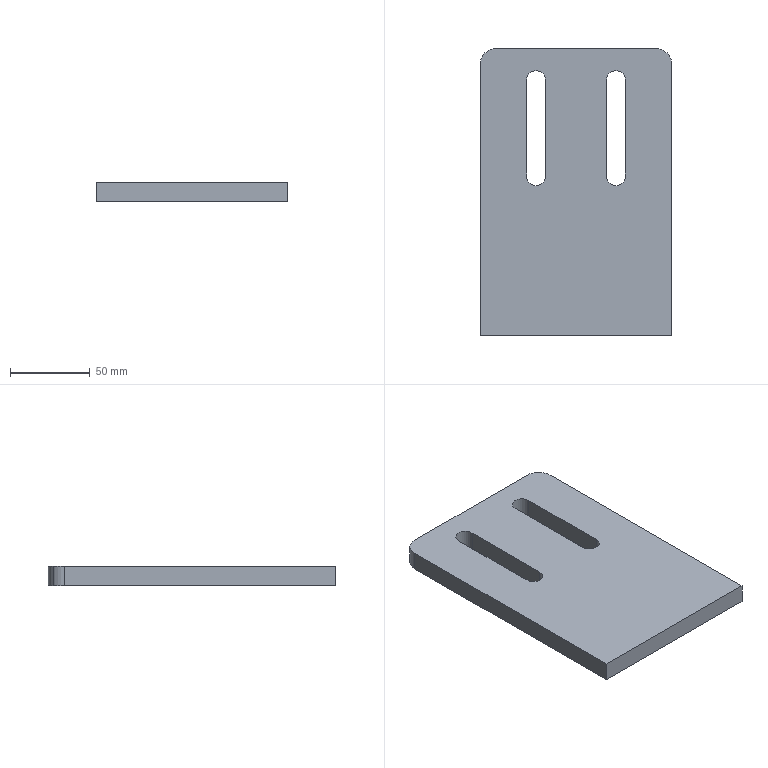Part | STEP file | DCV-000-021 | 1 solid | 18 faces | box 120 x 180 x 12 mm | volume 238691 mm3 | plane 10 | cylinder 8 | commonest cylinder face diameters 12 x4 20 x4
STEP:
#1=CARTESIAN_POINT('',(0.,0.,0.));
#2=DIRECTION('',(0.,0.,1.));
#3=DIRECTION('',(1.,0.,0.));
#4=AXIS2_PLACEMENT_3D('',#1,#2,#3);
#5=CARTESIAN_POINT('',(60.,170.,0.));
#6=VERTEX_POINT('',#5);
#7=CARTESIAN_POINT('',(57.071,177.071,0.));
#8=VERTEX_POINT('',#7);
#9=CARTESIAN_POINT('',(50.,170.,0.));
#10=DIRECTION('',(0.,0.,1.));
#11=DIRECTION('',(0.7071,0.7071,0.));
#12=AXIS2_PLACEMENT_3D('',#9,#10,#11);
#13=CIRCLE('',#12,10.);
#14=CARTESIAN_POINT('',(50.,170.,0.));
#15=DIRECTION('',(0.,0.,1.));
#16=DIRECTION('',(0.7071,0.7071,0.));
#17=AXIS2_PLACEMENT_3D('',#14,#15,#16);
#18=CYLINDRICAL_SURFACE('',#17,10.);
#19=CARTESIAN_POINT('',(0.,0.));
#20=DIRECTION('',(1.,0.));
#21=VECTOR('',#20,1.);
#22=LINE('',#19,#21);
#23=(GEOMETRIC_REPRESENTATION_CONTEXT(2)PARAMETRIC_REPRESENTATION_CONTEXT()REPRESENTATION_CONTEXT('',''));
#24=DEFINITIONAL_REPRESENTATION('',(#22),#23);
#25=PCURVE('',#18,#24);
#26=CARTESIAN_POINT('',(0.,90.,0.));
#27=DIRECTION('',(0.,0.,1.));
#28=DIRECTION('',(1.,0.,0.));
#29=AXIS2_PLACEMENT_3D('',#26,#27,#28);
#30=PLANE('',#29);
#31=CARTESIAN_POINT('',(50.,80.));
#32=DIRECTION('',(0.7071,0.7071));
#33=AXIS2_PLACEMENT_2D('',#31,#32);
#34=CIRCLE('',#33,10.);
#35=(GEOMETRIC_REPRESENTATION_CONTEXT(2)PARAMETRIC_REPRESENTATION_CONTEXT()REPRESENTATION_CONTEXT('',''));
#36=DEFINITIONAL_REPRESENTATION('',(#34),#35);
#37=PCURVE('',#30,#36);
#38=SURFACE_CURVE('',#13,(#25,#37),.PCURVE_S1.);
#39=EDGE_CURVE('',#6,#8,#38,.T.);
#40=ORIENTED_EDGE('',*,*,#39,.T.);
#41=CARTESIAN_POINT('',(57.071,177.071,12.));
#42=VERTEX_POINT('',#41);
#43=CARTESIAN_POINT('',(57.071,177.071,0.));
#44=DIRECTION('',(0.,0.,1.));
#45=VECTOR('',#44,1.);
#46=LINE('',#43,#45);
#47=CARTESIAN_POINT('',(6.283,0.));
#48=DIRECTION('',(0.,1.));
#49=VECTOR('',#48,1.);
#50=LINE('',#47,#49);
#51=(GEOMETRIC_REPRESENTATION_CONTEXT(2)PARAMETRIC_REPRESENTATION_CONTEXT()REPRESENTATION_CONTEXT('',''));
#52=DEFINITIONAL_REPRESENTATION('',(#50),#51);
#53=PCURVE('',#18,#52);
#54=CARTESIAN_POINT('',(50.,170.,0.));
#55=DIRECTION('',(0.,0.,1.));
#56=DIRECTION('',(0.7071,0.7071,0.));
#57=AXIS2_PLACEMENT_3D('',#54,#55,#56);
#58=CYLINDRICAL_SURFACE('',#57,10.);
#59=CARTESIAN_POINT('',(0.,0.));
#60=DIRECTION('',(0.,1.));
#61=VECTOR('',#60,1.);
#62=LINE('',#59,#61);
#63=(GEOMETRIC_REPRESENTATION_CONTEXT(2)PARAMETRIC_REPRESENTATION_CONTEXT()REPRESENTATION_CONTEXT('',''));
#64=DEFINITIONAL_REPRESENTATION('',(#62),#63);
#65=PCURVE('',#58,#64);
#66=SURFACE_CURVE('',#46,(#53,#65),.PCURVE_S1.);
#67=EDGE_CURVE('',#8,#42,#66,.T.);
#68=ORIENTED_EDGE('',*,*,#67,.T.);
#69=CARTESIAN_POINT('',(60.,170.,12.));
#70=VERTEX_POINT('',#69);
#71=CARTESIAN_POINT('',(50.,170.,12.));
#72=DIRECTION('',(0.,0.,-1.));
#73=DIRECTION('',(0.7071,0.7071,0.));
#74=AXIS2_PLACEMENT_3D('',#71,#72,#73);
#75=CIRCLE('',#74,10.);
#76=CARTESIAN_POINT('',(6.283,12.));
#77=DIRECTION('',(-1.,0.));
#78=VECTOR('',#77,1.);
#79=LINE('',#76,#78);
#80=(GEOMETRIC_REPRESENTATION_CONTEXT(2)PARAMETRIC_REPRESENTATION_CONTEXT()REPRESENTATION_CONTEXT('',''));
#81=DEFINITIONAL_REPRESENTATION('',(#79),#80);
#82=PCURVE('',#18,#81);
#83=CARTESIAN_POINT('',(0.,90.,12.));
#84=DIRECTION('',(0.,0.,1.));
#85=DIRECTION('',(1.,0.,0.));
#86=AXIS2_PLACEMENT_3D('',#83,#84,#85);
#87=PLANE('',#86);
#88=CARTESIAN_POINT('',(57.071,87.071));
#89=CARTESIAN_POINT('',(69.319,74.824));
#90=CARTESIAN_POINT('',(52.588,70.341));
#91=CARTESIAN_POINT('',(35.858,65.858));
#92=CARTESIAN_POINT('',(40.341,82.588));
#93=CARTESIAN_POINT('',(44.824,99.319));
#94=CARTESIAN_POINT('',(57.071,87.071));
#95=(BOUNDED_CURVE()B_SPLINE_CURVE(2,(#88,#89,#90,#91,#92,#93,#94),.UNSPECIFIED.,.T.,.F.)B_SPLINE_CURVE_WITH_KNOTS((1,2,2,2,2,1),(-2.094,0.,2.094,4.189,6.283,8.378),.UNSPECIFIED.)CURVE()GEOMETRIC_REPRESENTATION_ITEM()RATIONAL_B_SPLINE_CURVE((1.,0.5,1.,0.5,1.,0.5,1.))REPRESENTATION_ITEM(''));
#96=(GEOMETRIC_REPRESENTATION_CONTEXT(2)PARAMETRIC_REPRESENTATION_CONTEXT()REPRESENTATION_CONTEXT('',''));
#97=DEFINITIONAL_REPRESENTATION('',(#95),#96);
#98=PCURVE('',#87,#97);
#99=SURFACE_CURVE('',#75,(#82,#98),.PCURVE_S1.);
#100=EDGE_CURVE('',#42,#70,#99,.T.);
#101=ORIENTED_EDGE('',*,*,#100,.T.);
#102=CARTESIAN_POINT('',(60.,170.,0.));
#103=DIRECTION('',(0.,0.,-1.));
#104=VECTOR('',#103,1.);
#105=LINE('',#102,#104);
#106=CARTESIAN_POINT('',(5.498,0.));
#107=DIRECTION('',(0.,-1.));
#108=VECTOR('',#107,1.);
#109=LINE('',#106,#108);
#110=(GEOMETRIC_REPRESENTATION_CONTEXT(2)PARAMETRIC_REPRESENTATION_CONTEXT()REPRESENTATION_CONTEXT('',''));
#111=DEFINITIONAL_REPRESENTATION('',(#109),#110);
#112=PCURVE('',#18,#111);
#113=CARTESIAN_POINT('',(60.,0.,0.));
#114=DIRECTION('',(1.,0.,0.));
#115=DIRECTION('',(0.,1.,0.));
#116=AXIS2_PLACEMENT_3D('',#113,#114,#115);
#117=PLANE('',#116);
#118=CARTESIAN_POINT('',(170.,0.));
#119=DIRECTION('',(0.,-1.));
#120=VECTOR('',#119,1.);
#121=LINE('',#118,#120);
#122=(GEOMETRIC_REPRESENTATION_CONTEXT(2)PARAMETRIC_REPRESENTATION_CONTEXT()REPRESENTATION_CONTEXT('',''));
#123=DEFINITIONAL_REPRESENTATION('',(#121),#122);
#124=PCURVE('',#117,#123);
#125=SURFACE_CURVE('',#105,(#112,#124),.PCURVE_S1.);
#126=EDGE_CURVE('',#70,#6,#125,.T.);
#127=ORIENTED_EDGE('',*,*,#126,.T.);
#128=EDGE_LOOP('',(#40,#68,#101,#127));
#129=FACE_BOUND('',#128,.T.);
#130=ADVANCED_FACE('',(#129),#18,.T.);
#131=CARTESIAN_POINT('',(-50.,180.,0.));
#132=VERTEX_POINT('',#131);
#133=CARTESIAN_POINT('',(-57.071,177.071,0.));
#134=VERTEX_POINT('',#133);
#135=CARTESIAN_POINT('',(-50.,170.,0.));
#136=DIRECTION('',(0.,0.,1.));
#137=DIRECTION('',(-0.7071,0.7071,0.));
#138=AXIS2_PLACEMENT_3D('',#135,#136,#137);
#139=CIRCLE('',#138,10.);
#140=CARTESIAN_POINT('',(-50.,170.,0.));
#141=DIRECTION('',(0.,0.,1.));
#142=DIRECTION('',(-0.7071,0.7071,0.));
#143=AXIS2_PLACEMENT_3D('',#140,#141,#142);
#144=CYLINDRICAL_SURFACE('',#143,10.);
#145=CARTESIAN_POINT('',(0.,0.));
#146=DIRECTION('',(1.,0.));
#147=VECTOR('',#146,1.);
#148=LINE('',#145,#147);
#149=(GEOMETRIC_REPRESENTATION_CONTEXT(2)PARAMETRIC_REPRESENTATION_CONTEXT()REPRESENTATION_CONTEXT('',''));
#150=DEFINITIONAL_REPRESENTATION('',(#148),#149);
#151=PCURVE('',#144,#150);
#152=CARTESIAN_POINT('',(-50.,80.));
#153=DIRECTION('',(-0.7071,0.7071));
#154=AXIS2_PLACEMENT_2D('',#152,#153);
#155=CIRCLE('',#154,10.);
#156=(GEOMETRIC_REPRESENTATION_CONTEXT(2)PARAMETRIC_REPRESENTATION_CONTEXT()REPRESENTATION_CONTEXT('',''));
#157=DEFINITIONAL_REPRESENTATION('',(#155),#156);
#158=PCURVE('',#30,#157);
#159=SURFACE_CURVE('',#139,(#151,#158),.PCURVE_S1.);
#160=EDGE_CURVE('',#132,#134,#159,.T.);
#161=ORIENTED_EDGE('',*,*,#160,.T.);
#162=CARTESIAN_POINT('',(-57.071,177.071,12.));
#163=VERTEX_POINT('',#162);
#164=CARTESIAN_POINT('',(-57.071,177.071,0.));
#165=DIRECTION('',(0.,0.,1.));
#166=VECTOR('',#165,1.);
#167=LINE('',#164,#166);
#168=CARTESIAN_POINT('',(6.283,0.));
#169=DIRECTION('',(0.,1.));
#170=VECTOR('',#169,1.);
#171=LINE('',#168,#170);
#172=(GEOMETRIC_REPRESENTATION_CONTEXT(2)PARAMETRIC_REPRESENTATION_CONTEXT()REPRESENTATION_CONTEXT('',''));
#173=DEFINITIONAL_REPRESENTATION('',(#171),#172);
#174=PCURVE('',#144,#173);
#175=CARTESIAN_POINT('',(-50.,170.,0.));
#176=DIRECTION('',(0.,0.,1.));
#177=DIRECTION('',(-0.7071,0.7071,0.));
#178=AXIS2_PLACEMENT_3D('',#175,#176,#177);
#179=CYLINDRICAL_SURFACE('',#178,10.);
#180=CARTESIAN_POINT('',(0.,0.));
#181=DIRECTION('',(0.,1.));
#182=VECTOR('',#181,1.);
#183=LINE('',#180,#182);
#184=(GEOMETRIC_REPRESENTATION_CONTEXT(2)PARAMETRIC_REPRESENTATION_CONTEXT()REPRESENTATION_CONTEXT('',''));
#185=DEFINITIONAL_REPRESENTATION('',(#183),#184);
#186=PCURVE('',#179,#185);
#187=SURFACE_CURVE('',#167,(#174,#186),.PCURVE_S1.);
#188=EDGE_CURVE('',#134,#163,#187,.T.);
#189=ORIENTED_EDGE('',*,*,#188,.T.);
#190=CARTESIAN_POINT('',(-50.,180.,12.));
#191=VERTEX_POINT('',#190);
#192=CARTESIAN_POINT('',(-50.,170.,12.));
#193=DIRECTION('',(0.,0.,-1.));
#194=DIRECTION('',(-0.7071,0.7071,0.));
#195=AXIS2_PLACEMENT_3D('',#192,#193,#194);
#196=CIRCLE('',#195,10.);
#197=CARTESIAN_POINT('',(6.283,12.));
#198=DIRECTION('',(-1.,0.));
#199=VECTOR('',#198,1.);
#200=LINE('',#197,#199);
#201=(GEOMETRIC_REPRESENTATION_CONTEXT(2)PARAMETRIC_REPRESENTATION_CONTEXT()REPRESENTATION_CONTEXT('',''));
#202=DEFINITIONAL_REPRESENTATION('',(#200),#201);
#203=PCURVE('',#144,#202);
#204=CARTESIAN_POINT('',(-57.071,87.071));
#205=CARTESIAN_POINT('',(-44.824,99.319));
#206=CARTESIAN_POINT('',(-40.341,82.588));
#207=CARTESIAN_POINT('',(-35.858,65.858));
#208=CARTESIAN_POINT('',(-52.588,70.341));
#209=CARTESIAN_POINT('',(-69.319,74.824));
#210=CARTESIAN_POINT('',(-57.071,87.071));
#211=(BOUNDED_CURVE()B_SPLINE_CURVE(2,(#204,#205,#206,#207,#208,#209,#210),.UNSPECIFIED.,.T.,.F.)B_SPLINE_CURVE_WITH_KNOTS((1,2,2,2,2,1),(-2.094,0.,2.094,4.189,6.283,8.378),.UNSPECIFIED.)CURVE()GEOMETRIC_REPRESENTATION_ITEM()RATIONAL_B_SPLINE_CURVE((1.,0.5,1.,0.5,1.,0.5,1.))REPRESENTATION_ITEM(''));
#212=(GEOMETRIC_REPRESENTATION_CONTEXT(2)PARAMETRIC_REPRESENTATION_CONTEXT()REPRESENTATION_CONTEXT('',''));
#213=DEFINITIONAL_REPRESENTATION('',(#211),#212);
#214=PCURVE('',#87,#213);
#215=SURFACE_CURVE('',#196,(#203,#214),.PCURVE_S1.);
#216=EDGE_CURVE('',#163,#191,#215,.T.);
#217=ORIENTED_EDGE('',*,*,#216,.T.);
#218=CARTESIAN_POINT('',(-50.,180.,0.));
#219=DIRECTION('',(0.,0.,-1.));
#220=VECTOR('',#219,1.);
#221=LINE('',#218,#220);
#222=CARTESIAN_POINT('',(5.498,0.));
#223=DIRECTION('',(0.,-1.));
#224=VECTOR('',#223,1.);
#225=LINE('',#222,#224);
#226=(GEOMETRIC_REPRESENTATION_CONTEXT(2)PARAMETRIC_REPRESENTATION_CONTEXT()REPRESENTATION_CONTEXT('',''));
#227=DEFINITIONAL_REPRESENTATION('',(#225),#226);
#228=PCURVE('',#144,#227);
#229=CARTESIAN_POINT('',(60.,180.,0.));
#230=DIRECTION('',(0.,1.,0.));
#231=DIRECTION('',(1.,0.,0.));
#232=AXIS2_PLACEMENT_3D('',#229,#230,#231);
#233=PLANE('',#232);
#234=CARTESIAN_POINT('',(-110.,0.));
#235=DIRECTION('',(0.,1.));
#236=VECTOR('',#235,1.);
#237=LINE('',#234,#236);
#238=(GEOMETRIC_REPRESENTATION_CONTEXT(2)PARAMETRIC_REPRESENTATION_CONTEXT()REPRESENTATION_CONTEXT('',''));
#239=DEFINITIONAL_REPRESENTATION('',(#237),#238);
#240=PCURVE('',#233,#239);
#241=SURFACE_CURVE('',#221,(#228,#240),.PCURVE_S1.);
#242=EDGE_CURVE('',#191,#132,#241,.T.);
#243=ORIENTED_EDGE('',*,*,#242,.T.);
#244=EDGE_LOOP('',(#161,#189,#217,#243));
#245=FACE_BOUND('',#244,.T.);
#246=ADVANCED_FACE('',(#245),#144,.T.);
#247=CARTESIAN_POINT('',(31.,160.,0.));
#248=VERTEX_POINT('',#247);
#249=CARTESIAN_POINT('',(31.,100.,0.));
#250=VERTEX_POINT('',#249);
#251=CARTESIAN_POINT('',(31.,160.,0.));
#252=DIRECTION('',(0.,-1.,0.));
#253=VECTOR('',#252,1.);
#254=LINE('',#251,#253);
#255=CARTESIAN_POINT('',(31.,70.));
#256=DIRECTION('',(0.,-1.));
#257=VECTOR('',#256,1.);
#258=LINE('',#255,#257);
#259=(GEOMETRIC_REPRESENTATION_CONTEXT(2)PARAMETRIC_REPRESENTATION_CONTEXT()REPRESENTATION_CONTEXT('',''));
#260=DEFINITIONAL_REPRESENTATION('',(#258),#259);
#261=PCURVE('',#30,#260);
#262=CARTESIAN_POINT('',(31.,160.,0.));
#263=DIRECTION('',(-1.,0.,0.));
#264=DIRECTION('',(0.,0.,1.));
#265=AXIS2_PLACEMENT_3D('',#262,#263,#264);
#266=PLANE('',#265);
#267=CARTESIAN_POINT('',(0.,0.));
#268=DIRECTION('',(0.,-1.));
#269=VECTOR('',#268,1.);
#270=LINE('',#267,#269);
#271=(GEOMETRIC_REPRESENTATION_CONTEXT(2)PARAMETRIC_REPRESENTATION_CONTEXT()REPRESENTATION_CONTEXT('',''));
#272=DEFINITIONAL_REPRESENTATION('',(#270),#271);
#273=PCURVE('',#266,#272);
#274=SURFACE_CURVE('',#254,(#261,#273),.PCURVE_S1.);
#275=EDGE_CURVE('',#248,#250,#274,.T.);
#276=ORIENTED_EDGE('',*,*,#275,.F.);
#277=CARTESIAN_POINT('',(19.,160.,0.));
#278=VERTEX_POINT('',#277);
#279=CARTESIAN_POINT('',(25.,160.,0.));
#280=DIRECTION('',(0.,0.,-1.));
#281=DIRECTION('',(-1.,0.,0.));
#282=AXIS2_PLACEMENT_3D('',#279,#280,#281);
#283=CIRCLE('',#282,6.);
#284=CARTESIAN_POINT('',(19.,70.));
#285=CARTESIAN_POINT('',(19.,80.392));
#286=CARTESIAN_POINT('',(28.,75.196));
#287=CARTESIAN_POINT('',(37.,70.));
#288=CARTESIAN_POINT('',(28.,64.804));
#289=CARTESIAN_POINT('',(19.,59.608));
#290=CARTESIAN_POINT('',(19.,70.));
#291=(BOUNDED_CURVE()B_SPLINE_CURVE(2,(#284,#285,#286,#287,#288,#289,#290),.UNSPECIFIED.,.T.,.F.)B_SPLINE_CURVE_WITH_KNOTS((1,2,2,2,2,1),(-2.094,0.,2.094,4.189,6.283,8.378),.UNSPECIFIED.)CURVE()GEOMETRIC_REPRESENTATION_ITEM()RATIONAL_B_SPLINE_CURVE((1.,0.5,1.,0.5,1.,0.5,1.))REPRESENTATION_ITEM(''));
#292=(GEOMETRIC_REPRESENTATION_CONTEXT(2)PARAMETRIC_REPRESENTATION_CONTEXT()REPRESENTATION_CONTEXT('',''));
#293=DEFINITIONAL_REPRESENTATION('',(#291),#292);
#294=PCURVE('',#30,#293);
#295=CARTESIAN_POINT('',(25.,160.,0.));
#296=DIRECTION('',(0.,0.,1.));
#297=DIRECTION('',(-1.,0.,0.));
#298=AXIS2_PLACEMENT_3D('',#295,#296,#297);
#299=CYLINDRICAL_SURFACE('',#298,6.);
#300=CARTESIAN_POINT('',(6.283,0.));
#301=DIRECTION('',(-1.,0.));
#302=VECTOR('',#301,1.);
#303=LINE('',#300,#302);
#304=(GEOMETRIC_REPRESENTATION_CONTEXT(2)PARAMETRIC_REPRESENTATION_CONTEXT()REPRESENTATION_CONTEXT('',''));
#305=DEFINITIONAL_REPRESENTATION('',(#303),#304);
#306=PCURVE('',#299,#305);
#307=SURFACE_CURVE('',#283,(#294,#306),.PCURVE_S1.);
#308=EDGE_CURVE('',#278,#248,#307,.T.);
#309=ORIENTED_EDGE('',*,*,#308,.F.);
#310=CARTESIAN_POINT('',(19.,100.,0.));
#311=VERTEX_POINT('',#310);
#312=CARTESIAN_POINT('',(19.,100.,0.));
#313=DIRECTION('',(0.,1.,0.));
#314=VECTOR('',#313,1.);
#315=LINE('',#312,#314);
#316=CARTESIAN_POINT('',(19.,10.));
#317=DIRECTION('',(0.,1.));
#318=VECTOR('',#317,1.);
#319=LINE('',#316,#318);
#320=(GEOMETRIC_REPRESENTATION_CONTEXT(2)PARAMETRIC_REPRESENTATION_CONTEXT()REPRESENTATION_CONTEXT('',''));
#321=DEFINITIONAL_REPRESENTATION('',(#319),#320);
#322=PCURVE('',#30,#321);
#323=CARTESIAN_POINT('',(19.,100.,0.));
#324=DIRECTION('',(1.,0.,0.));
#325=DIRECTION('',(0.,1.,0.));
#326=AXIS2_PLACEMENT_3D('',#323,#324,#325);
#327=PLANE('',#326);
#328=CARTESIAN_POINT('',(0.,0.));
#329=DIRECTION('',(1.,0.));
#330=VECTOR('',#329,1.);
#331=LINE('',#328,#330);
#332=(GEOMETRIC_REPRESENTATION_CONTEXT(2)PARAMETRIC_REPRESENTATION_CONTEXT()REPRESENTATION_CONTEXT('',''));
#333=DEFINITIONAL_REPRESENTATION('',(#331),#332);
#334=PCURVE('',#327,#333);
#335=SURFACE_CURVE('',#315,(#322,#334),.PCURVE_S1.);
#336=EDGE_CURVE('',#311,#278,#335,.T.);
#337=ORIENTED_EDGE('',*,*,#336,.F.);
#338=CARTESIAN_POINT('',(25.,100.,0.));
#339=DIRECTION('',(0.,0.,-1.));
#340=DIRECTION('',(1.,0.,0.));
#341=AXIS2_PLACEMENT_3D('',#338,#339,#340);
#342=CIRCLE('',#341,6.);
#343=CARTESIAN_POINT('',(31.,10.));
#344=CARTESIAN_POINT('',(31.,-0.3923));
#345=CARTESIAN_POINT('',(22.,4.804));
#346=CARTESIAN_POINT('',(13.,10.));
#347=CARTESIAN_POINT('',(22.,15.196));
#348=CARTESIAN_POINT('',(31.,20.392));
#349=CARTESIAN_POINT('',(31.,10.));
#350=(BOUNDED_CURVE()B_SPLINE_CURVE(2,(#343,#344,#345,#346,#347,#348,#349),.UNSPECIFIED.,.T.,.F.)B_SPLINE_CURVE_WITH_KNOTS((1,2,2,2,2,1),(-2.094,0.,2.094,4.189,6.283,8.378),.UNSPECIFIED.)CURVE()GEOMETRIC_REPRESENTATION_ITEM()RATIONAL_B_SPLINE_CURVE((1.,0.5,1.,0.5,1.,0.5,1.))REPRESENTATION_ITEM(''));
#351=(GEOMETRIC_REPRESENTATION_CONTEXT(2)PARAMETRIC_REPRESENTATION_CONTEXT()REPRESENTATION_CONTEXT('',''));
#352=DEFINITIONAL_REPRESENTATION('',(#350),#351);
#353=PCURVE('',#30,#352);
#354=CARTESIAN_POINT('',(25.,100.,0.));
#355=DIRECTION('',(0.,0.,1.));
#356=DIRECTION('',(1.,0.,0.));
#357=AXIS2_PLACEMENT_3D('',#354,#355,#356);
#358=CYLINDRICAL_SURFACE('',#357,6.);
#359=CARTESIAN_POINT('',(6.283,0.));
#360=DIRECTION('',(-1.,0.));
#361=VECTOR('',#360,1.);
#362=LINE('',#359,#361);
#363=(GEOMETRIC_REPRESENTATION_CONTEXT(2)PARAMETRIC_REPRESENTATION_CONTEXT()REPRESENTATION_CONTEXT('',''));
#364=DEFINITIONAL_REPRESENTATION('',(#362),#363);
#365=PCURVE('',#358,#364);
#366=SURFACE_CURVE('',#342,(#353,#365),.PCURVE_S1.);
#367=EDGE_CURVE('',#250,#311,#366,.T.);
#368=ORIENTED_EDGE('',*,*,#367,.F.);
#369=EDGE_LOOP('',(#276,#309,#337,#368));
#370=FACE_BOUND('',#369,.T.);
#371=CARTESIAN_POINT('',(-31.,100.,0.));
#372=VERTEX_POINT('',#371);
#373=CARTESIAN_POINT('',(-31.,160.,0.));
#374=VERTEX_POINT('',#373);
#375=CARTESIAN_POINT('',(-31.,100.,0.));
#376=DIRECTION('',(0.,1.,0.));
#377=VECTOR('',#376,1.);
#378=LINE('',#375,#377);
#379=CARTESIAN_POINT('',(-31.,10.));
#380=DIRECTION('',(0.,1.));
#381=VECTOR('',#380,1.);
#382=LINE('',#379,#381);
#383=(GEOMETRIC_REPRESENTATION_CONTEXT(2)PARAMETRIC_REPRESENTATION_CONTEXT()REPRESENTATION_CONTEXT('',''));
#384=DEFINITIONAL_REPRESENTATION('',(#382),#383);
#385=PCURVE('',#30,#384);
#386=CARTESIAN_POINT('',(-31.,100.,0.));
#387=DIRECTION('',(1.,0.,0.));
#388=DIRECTION('',(0.,1.,0.));
#389=AXIS2_PLACEMENT_3D('',#386,#387,#388);
#390=PLANE('',#389);
#391=CARTESIAN_POINT('',(0.,0.));
#392=DIRECTION('',(1.,0.));
#393=VECTOR('',#392,1.);
#394=LINE('',#391,#393);
#395=(GEOMETRIC_REPRESENTATION_CONTEXT(2)PARAMETRIC_REPRESENTATION_CONTEXT()REPRESENTATION_CONTEXT('',''));
#396=DEFINITIONAL_REPRESENTATION('',(#394),#395);
#397=PCURVE('',#390,#396);
#398=SURFACE_CURVE('',#378,(#385,#397),.PCURVE_S1.);
#399=EDGE_CURVE('',#372,#374,#398,.T.);
#400=ORIENTED_EDGE('',*,*,#399,.F.);
#401=CARTESIAN_POINT('',(-19.,100.,0.));
#402=VERTEX_POINT('',#401);
#403=CARTESIAN_POINT('',(-25.,100.,0.));
#404=DIRECTION('',(0.,0.,-1.));
#405=DIRECTION('',(1.,0.,0.));
#406=AXIS2_PLACEMENT_3D('',#403,#404,#405);
#407=CIRCLE('',#406,6.);
#408=CARTESIAN_POINT('',(-19.,10.));
#409=CARTESIAN_POINT('',(-19.,-0.3923));
#410=CARTESIAN_POINT('',(-28.,4.804));
#411=CARTESIAN_POINT('',(-37.,10.));
#412=CARTESIAN_POINT('',(-28.,15.196));
#413=CARTESIAN_POINT('',(-19.,20.392));
#414=CARTESIAN_POINT('',(-19.,10.));
#415=(BOUNDED_CURVE()B_SPLINE_CURVE(2,(#408,#409,#410,#411,#412,#413,#414),.UNSPECIFIED.,.T.,.F.)B_SPLINE_CURVE_WITH_KNOTS((1,2,2,2,2,1),(-2.094,0.,2.094,4.189,6.283,8.378),.UNSPECIFIED.)CURVE()GEOMETRIC_REPRESENTATION_ITEM()RATIONAL_B_SPLINE_CURVE((1.,0.5,1.,0.5,1.,0.5,1.))REPRESENTATION_ITEM(''));
#416=(GEOMETRIC_REPRESENTATION_CONTEXT(2)PARAMETRIC_REPRESENTATION_CONTEXT()REPRESENTATION_CONTEXT('',''));
#417=DEFINITIONAL_REPRESENTATION('',(#415),#416);
#418=PCURVE('',#30,#417);
#419=CARTESIAN_POINT('',(-25.,100.,0.));
#420=DIRECTION('',(0.,0.,1.));
#421=DIRECTION('',(1.,0.,0.));
#422=AXIS2_PLACEMENT_3D('',#419,#420,#421);
#423=CYLINDRICAL_SURFACE('',#422,6.);
#424=CARTESIAN_POINT('',(6.283,0.));
#425=DIRECTION('',(-1.,0.));
#426=VECTOR('',#425,1.);
#427=LINE('',#424,#426);
#428=(GEOMETRIC_REPRESENTATION_CONTEXT(2)PARAMETRIC_REPRESENTATION_CONTEXT()REPRESENTATION_CONTEXT('',''));
#429=DEFINITIONAL_REPRESENTATION('',(#427),#428);
#430=PCURVE('',#423,#429);
#431=SURFACE_CURVE('',#407,(#418,#430),.PCURVE_S1.);
#432=EDGE_CURVE('',#402,#372,#431,.T.);
#433=ORIENTED_EDGE('',*,*,#432,.F.);
#434=CARTESIAN_POINT('',(-19.,160.,0.));
#435=VERTEX_POINT('',#434);
#436=CARTESIAN_POINT('',(-19.,160.,0.));
#437=DIRECTION('',(0.,-1.,0.));
#438=VECTOR('',#437,1.);
#439=LINE('',#436,#438);
#440=CARTESIAN_POINT('',(-19.,70.));
#441=DIRECTION('',(0.,-1.));
#442=VECTOR('',#441,1.);
#443=LINE('',#440,#442);
#444=(GEOMETRIC_REPRESENTATION_CONTEXT(2)PARAMETRIC_REPRESENTATION_CONTEXT()REPRESENTATION_CONTEXT('',''));
#445=DEFINITIONAL_REPRESENTATION('',(#443),#444);
#446=PCURVE('',#30,#445);
#447=CARTESIAN_POINT('',(-19.,160.,0.));
#448=DIRECTION('',(-1.,0.,0.));
#449=DIRECTION('',(0.,1.,0.));
#450=AXIS2_PLACEMENT_3D('',#447,#448,#449);
#451=PLANE('',#450);
#452=CARTESIAN_POINT('',(0.,0.));
#453=DIRECTION('',(-1.,0.));
#454=VECTOR('',#453,1.);
#455=LINE('',#452,#454);
#456=(GEOMETRIC_REPRESENTATION_CONTEXT(2)PARAMETRIC_REPRESENTATION_CONTEXT()REPRESENTATION_CONTEXT('',''));
#457=DEFINITIONAL_REPRESENTATION('',(#455),#456);
#458=PCURVE('',#451,#457);
#459=SURFACE_CURVE('',#439,(#446,#458),.PCURVE_S1.);
#460=EDGE_CURVE('',#435,#402,#459,.T.);
#461=ORIENTED_EDGE('',*,*,#460,.F.);
#462=CARTESIAN_POINT('',(-25.,160.,0.));
#463=DIRECTION('',(0.,0.,-1.));
#464=DIRECTION('',(-1.,0.,0.));
#465=AXIS2_PLACEMENT_3D('',#462,#463,#464);
#466=CIRCLE('',#465,6.);
#467=CARTESIAN_POINT('',(-31.,70.));
#468=CARTESIAN_POINT('',(-31.,80.392));
#469=CARTESIAN_POINT('',(-22.,75.196));
#470=CARTESIAN_POINT('',(-13.,70.));
#471=CARTESIAN_POINT('',(-22.,64.804));
#472=CARTESIAN_POINT('',(-31.,59.608));
#473=CARTESIAN_POINT('',(-31.,70.));
#474=(BOUNDED_CURVE()B_SPLINE_CURVE(2,(#467,#468,#469,#470,#471,#472,#473),.UNSPECIFIED.,.T.,.F.)B_SPLINE_CURVE_WITH_KNOTS((1,2,2,2,2,1),(-2.094,0.,2.094,4.189,6.283,8.378),.UNSPECIFIED.)CURVE()GEOMETRIC_REPRESENTATION_ITEM()RATIONAL_B_SPLINE_CURVE((1.,0.5,1.,0.5,1.,0.5,1.))REPRESENTATION_ITEM(''));
#475=(GEOMETRIC_REPRESENTATION_CONTEXT(2)PARAMETRIC_REPRESENTATION_CONTEXT()REPRESENTATION_CONTEXT('',''));
#476=DEFINITIONAL_REPRESENTATION('',(#474),#475);
#477=PCURVE('',#30,#476);
#478=CARTESIAN_POINT('',(-25.,160.,0.));
#479=DIRECTION('',(0.,0.,1.));
#480=DIRECTION('',(-1.,0.,0.));
#481=AXIS2_PLACEMENT_3D('',#478,#479,#480);
#482=CYLINDRICAL_SURFACE('',#481,6.);
#483=CARTESIAN_POINT('',(6.283,0.));
#484=DIRECTION('',(-1.,0.));
#485=VECTOR('',#484,1.);
#486=LINE('',#483,#485);
#487=(GEOMETRIC_REPRESENTATION_CONTEXT(2)PARAMETRIC_REPRESENTATION_CONTEXT()REPRESENTATION_CONTEXT('',''));
#488=DEFINITIONAL_REPRESENTATION('',(#486),#487);
#489=PCURVE('',#482,#488);
#490=SURFACE_CURVE('',#466,(#477,#489),.PCURVE_S1.);
#491=EDGE_CURVE('',#374,#435,#490,.T.);
#492=ORIENTED_EDGE('',*,*,#491,.F.);
#493=EDGE_LOOP('',(#400,#433,#461,#492));
#494=FACE_BOUND('',#493,.T.);
#495=ORIENTED_EDGE('',*,*,#39,.F.);
#496=CARTESIAN_POINT('',(60.,0.,0.));
#497=VERTEX_POINT('',#496);
#498=CARTESIAN_POINT('',(60.,0.,0.));
#499=DIRECTION('',(0.,1.,0.));
#500=VECTOR('',#499,1.);
#501=LINE('',#498,#500);
#502=CARTESIAN_POINT('',(60.,-90.));
#503=DIRECTION('',(0.,1.));
#504=VECTOR('',#503,1.);
#505=LINE('',#502,#504);
#506=(GEOMETRIC_REPRESENTATION_CONTEXT(2)PARAMETRIC_REPRESENTATION_CONTEXT()REPRESENTATION_CONTEXT('',''));
#507=DEFINITIONAL_REPRESENTATION('',(#505),#506);
#508=PCURVE('',#30,#507);
#509=CARTESIAN_POINT('',(0.,0.));
#510=DIRECTION('',(1.,0.));
#511=VECTOR('',#510,1.);
#512=LINE('',#509,#511);
#513=(GEOMETRIC_REPRESENTATION_CONTEXT(2)PARAMETRIC_REPRESENTATION_CONTEXT()REPRESENTATION_CONTEXT('',''));
#514=DEFINITIONAL_REPRESENTATION('',(#512),#513);
#515=PCURVE('',#117,#514);
#516=SURFACE_CURVE('',#501,(#508,#515),.PCURVE_S1.);
#517=EDGE_CURVE('',#497,#6,#516,.T.);
#518=ORIENTED_EDGE('',*,*,#517,.F.);
#519=CARTESIAN_POINT('',(-60.,0.,0.));
#520=VERTEX_POINT('',#519);
#521=CARTESIAN_POINT('',(-60.,0.,0.));
#522=DIRECTION('',(1.,0.,0.));
#523=VECTOR('',#522,1.);
#524=LINE('',#521,#523);
#525=CARTESIAN_POINT('',(-60.,-90.));
#526=DIRECTION('',(1.,0.));
#527=VECTOR('',#526,1.);
#528=LINE('',#525,#527);
#529=(GEOMETRIC_REPRESENTATION_CONTEXT(2)PARAMETRIC_REPRESENTATION_CONTEXT()REPRESENTATION_CONTEXT('',''));
#530=DEFINITIONAL_REPRESENTATION('',(#528),#529);
#531=PCURVE('',#30,#530);
#532=CARTESIAN_POINT('',(-60.,0.,0.));
#533=DIRECTION('',(0.,-1.,0.));
#534=DIRECTION('',(0.,0.,-1.));
#535=AXIS2_PLACEMENT_3D('',#532,#533,#534);
#536=PLANE('',#535);
#537=CARTESIAN_POINT('',(0.,0.));
#538=DIRECTION('',(0.,1.));
#539=VECTOR('',#538,1.);
#540=LINE('',#537,#539);
#541=(GEOMETRIC_REPRESENTATION_CONTEXT(2)PARAMETRIC_REPRESENTATION_CONTEXT()REPRESENTATION_CONTEXT('',''));
#542=DEFINITIONAL_REPRESENTATION('',(#540),#541);
#543=PCURVE('',#536,#542);
#544=SURFACE_CURVE('',#524,(#531,#543),.PCURVE_S1.);
#545=EDGE_CURVE('',#520,#497,#544,.T.);
#546=ORIENTED_EDGE('',*,*,#545,.F.);
#547=CARTESIAN_POINT('',(-60.,170.,0.));
#548=VERTEX_POINT('',#547);
#549=CARTESIAN_POINT('',(-60.,180.,0.));
#550=DIRECTION('',(0.,-1.,0.));
#551=VECTOR('',#550,1.);
#552=LINE('',#549,#551);
#553=CARTESIAN_POINT('',(-60.,90.));
#554=DIRECTION('',(0.,-1.));
#555=VECTOR('',#554,1.);
#556=LINE('',#553,#555);
#557=(GEOMETRIC_REPRESENTATION_CONTEXT(2)PARAMETRIC_REPRESENTATION_CONTEXT()REPRESENTATION_CONTEXT('',''));
#558=DEFINITIONAL_REPRESENTATION('',(#556),#557);
#559=PCURVE('',#30,#558);
#560=CARTESIAN_POINT('',(-60.,180.,0.));
#561=DIRECTION('',(-1.,0.,0.));
#562=DIRECTION('',(0.,1.,0.));
#563=AXIS2_PLACEMENT_3D('',#560,#561,#562);
#564=PLANE('',#563);
#565=CARTESIAN_POINT('',(0.,0.));
#566=DIRECTION('',(-1.,0.));
#567=VECTOR('',#566,1.);
#568=LINE('',#565,#567);
#569=(GEOMETRIC_REPRESENTATION_CONTEXT(2)PARAMETRIC_REPRESENTATION_CONTEXT()REPRESENTATION_CONTEXT('',''));
#570=DEFINITIONAL_REPRESENTATION('',(#568),#569);
#571=PCURVE('',#564,#570);
#572=SURFACE_CURVE('',#552,(#559,#571),.PCURVE_S1.);
#573=EDGE_CURVE('',#548,#520,#572,.T.);
#574=ORIENTED_EDGE('',*,*,#573,.F.);
#575=CARTESIAN_POINT('',(-50.,170.,0.));
#576=DIRECTION('',(0.,0.,1.));
#577=DIRECTION('',(-0.7071,0.7071,0.));
#578=AXIS2_PLACEMENT_3D('',#575,#576,#577);
#579=CIRCLE('',#578,10.);
#580=CARTESIAN_POINT('',(-50.,80.));
#581=DIRECTION('',(-0.7071,0.7071));
#582=AXIS2_PLACEMENT_2D('',#580,#581);
#583=CIRCLE('',#582,10.);
#584=(GEOMETRIC_REPRESENTATION_CONTEXT(2)PARAMETRIC_REPRESENTATION_CONTEXT()REPRESENTATION_CONTEXT('',''));
#585=DEFINITIONAL_REPRESENTATION('',(#583),#584);
#586=PCURVE('',#30,#585);
#587=CARTESIAN_POINT('',(0.,0.));
#588=DIRECTION('',(1.,0.));
#589=VECTOR('',#588,1.);
#590=LINE('',#587,#589);
#591=(GEOMETRIC_REPRESENTATION_CONTEXT(2)PARAMETRIC_REPRESENTATION_CONTEXT()REPRESENTATION_CONTEXT('',''));
#592=DEFINITIONAL_REPRESENTATION('',(#590),#591);
#593=PCURVE('',#179,#592);
#594=SURFACE_CURVE('',#579,(#586,#593),.PCURVE_S1.);
#595=EDGE_CURVE('',#134,#548,#594,.T.);
#596=ORIENTED_EDGE('',*,*,#595,.F.);
#597=ORIENTED_EDGE('',*,*,#160,.F.);
#598=CARTESIAN_POINT('',(50.,180.,0.));
#599=VERTEX_POINT('',#598);
#600=CARTESIAN_POINT('',(60.,180.,0.));
#601=DIRECTION('',(-1.,0.,0.));
#602=VECTOR('',#601,1.);
#603=LINE('',#600,#602);
#604=CARTESIAN_POINT('',(60.,90.));
#605=DIRECTION('',(-1.,0.));
#606=VECTOR('',#605,1.);
#607=LINE('',#604,#606);
#608=(GEOMETRIC_REPRESENTATION_CONTEXT(2)PARAMETRIC_REPRESENTATION_CONTEXT()REPRESENTATION_CONTEXT('',''));
#609=DEFINITIONAL_REPRESENTATION('',(#607),#608);
#610=PCURVE('',#30,#609);
#611=CARTESIAN_POINT('',(0.,0.));
#612=DIRECTION('',(-1.,0.));
#613=VECTOR('',#612,1.);
#614=LINE('',#611,#613);
#615=(GEOMETRIC_REPRESENTATION_CONTEXT(2)PARAMETRIC_REPRESENTATION_CONTEXT()REPRESENTATION_CONTEXT('',''));
#616=DEFINITIONAL_REPRESENTATION('',(#614),#615);
#617=PCURVE('',#233,#616);
#618=SURFACE_CURVE('',#603,(#610,#617),.PCURVE_S1.);
#619=EDGE_CURVE('',#599,#132,#618,.T.);
#620=ORIENTED_EDGE('',*,*,#619,.F.);
#621=CARTESIAN_POINT('',(50.,170.,0.));
#622=DIRECTION('',(0.,0.,1.));
#623=DIRECTION('',(0.7071,0.7071,0.));
#624=AXIS2_PLACEMENT_3D('',#621,#622,#623);
#625=CIRCLE('',#624,10.);
#626=CARTESIAN_POINT('',(50.,80.));
#627=DIRECTION('',(0.7071,0.7071));
#628=AXIS2_PLACEMENT_2D('',#626,#627);
#629=CIRCLE('',#628,10.);
#630=(GEOMETRIC_REPRESENTATION_CONTEXT(2)PARAMETRIC_REPRESENTATION_CONTEXT()REPRESENTATION_CONTEXT('',''));
#631=DEFINITIONAL_REPRESENTATION('',(#629),#630);
#632=PCURVE('',#30,#631);
#633=CARTESIAN_POINT('',(0.,0.));
#634=DIRECTION('',(1.,0.));
#635=VECTOR('',#634,1.);
#636=LINE('',#633,#635);
#637=(GEOMETRIC_REPRESENTATION_CONTEXT(2)PARAMETRIC_REPRESENTATION_CONTEXT()REPRESENTATION_CONTEXT('',''));
#638=DEFINITIONAL_REPRESENTATION('',(#636),#637);
#639=PCURVE('',#58,#638);
#640=SURFACE_CURVE('',#625,(#632,#639),.PCURVE_S1.);
#641=EDGE_CURVE('',#8,#599,#640,.T.);
#642=ORIENTED_EDGE('',*,*,#641,.F.);
#643=EDGE_LOOP('',(#495,#518,#546,#574,#596,#597,#620,#642));
#644=FACE_BOUND('',#643,.T.);
#645=ADVANCED_FACE('',(#370,#494,#644),#30,.F.);
#646=ORIENTED_EDGE('',*,*,#545,.T.);
#647=CARTESIAN_POINT('',(60.,0.,12.));
#648=VERTEX_POINT('',#647);
#649=CARTESIAN_POINT('',(60.,0.,0.));
#650=DIRECTION('',(0.,0.,1.));
#651=VECTOR('',#650,1.);
#652=LINE('',#649,#651);
#653=CARTESIAN_POINT('',(0.,120.));
#654=DIRECTION('',(-1.,0.));
#655=VECTOR('',#654,1.);
#656=LINE('',#653,#655);
#657=(GEOMETRIC_REPRESENTATION_CONTEXT(2)PARAMETRIC_REPRESENTATION_CONTEXT()REPRESENTATION_CONTEXT('',''));
#658=DEFINITIONAL_REPRESENTATION('',(#656),#657);
#659=PCURVE('',#536,#658);
#660=CARTESIAN_POINT('',(0.,0.));
#661=DIRECTION('',(0.,1.));
#662=VECTOR('',#661,1.);
#663=LINE('',#660,#662);
#664=(GEOMETRIC_REPRESENTATION_CONTEXT(2)PARAMETRIC_REPRESENTATION_CONTEXT()REPRESENTATION_CONTEXT('',''));
#665=DEFINITIONAL_REPRESENTATION('',(#663),#664);
#666=PCURVE('',#117,#665);
#667=SURFACE_CURVE('',#652,(#659,#666),.PCURVE_S1.);
#668=EDGE_CURVE('',#497,#648,#667,.T.);
#669=ORIENTED_EDGE('',*,*,#668,.T.);
#670=CARTESIAN_POINT('',(-60.,0.,12.));
#671=VERTEX_POINT('',#670);
#672=CARTESIAN_POINT('',(-60.,0.,12.));
#673=DIRECTION('',(1.,0.,0.));
#674=VECTOR('',#673,1.);
#675=LINE('',#672,#674);
#676=CARTESIAN_POINT('',(-12.,0.));
#677=DIRECTION('',(0.,1.));
#678=VECTOR('',#677,1.);
#679=LINE('',#676,#678);
#680=(GEOMETRIC_REPRESENTATION_CONTEXT(2)PARAMETRIC_REPRESENTATION_CONTEXT()REPRESENTATION_CONTEXT('',''));
#681=DEFINITIONAL_REPRESENTATION('',(#679),#680);
#682=PCURVE('',#536,#681);
#683=CARTESIAN_POINT('',(-60.,-90.));
#684=DIRECTION('',(1.,0.));
#685=VECTOR('',#684,1.);
#686=LINE('',#683,#685);
#687=(GEOMETRIC_REPRESENTATION_CONTEXT(2)PARAMETRIC_REPRESENTATION_CONTEXT()REPRESENTATION_CONTEXT('',''));
#688=DEFINITIONAL_REPRESENTATION('',(#686),#687);
#689=PCURVE('',#87,#688);
#690=SURFACE_CURVE('',#675,(#682,#689),.PCURVE_S1.);
#691=EDGE_CURVE('',#671,#648,#690,.T.);
#692=ORIENTED_EDGE('',*,*,#691,.F.);
#693=CARTESIAN_POINT('',(-60.,0.,0.));
#694=DIRECTION('',(0.,0.,1.));
#695=VECTOR('',#694,1.);
#696=LINE('',#693,#695);
#697=CARTESIAN_POINT('',(0.,0.));
#698=DIRECTION('',(-1.,0.));
#699=VECTOR('',#698,1.);
#700=LINE('',#697,#699);
#701=(GEOMETRIC_REPRESENTATION_CONTEXT(2)PARAMETRIC_REPRESENTATION_CONTEXT()REPRESENTATION_CONTEXT('',''));
#702=DEFINITIONAL_REPRESENTATION('',(#700),#701);
#703=PCURVE('',#536,#702);
#704=CARTESIAN_POINT('',(-180.,0.));
#705=DIRECTION('',(0.,-1.));
#706=VECTOR('',#705,1.);
#707=LINE('',#704,#706);
#708=(GEOMETRIC_REPRESENTATION_CONTEXT(2)PARAMETRIC_REPRESENTATION_CONTEXT()REPRESENTATION_CONTEXT('',''));
#709=DEFINITIONAL_REPRESENTATION('',(#707),#708);
#710=PCURVE('',#564,#709);
#711=SURFACE_CURVE('',#696,(#703,#710),.PCURVE_S1.);
#712=EDGE_CURVE('',#520,#671,#711,.T.);
#713=ORIENTED_EDGE('',*,*,#712,.F.);
#714=EDGE_LOOP('',(#646,#669,#692,#713));
#715=FACE_BOUND('',#714,.T.);
#716=ADVANCED_FACE('',(#715),#536,.T.);
#717=CARTESIAN_POINT('',(50.,180.,12.));
#718=VERTEX_POINT('',#717);
#719=CARTESIAN_POINT('',(50.,180.,0.));
#720=DIRECTION('',(0.,0.,1.));
#721=VECTOR('',#720,1.);
#722=LINE('',#719,#721);
#723=CARTESIAN_POINT('',(-10.,0.));
#724=DIRECTION('',(0.,-1.));
#725=VECTOR('',#724,1.);
#726=LINE('',#723,#725);
#727=(GEOMETRIC_REPRESENTATION_CONTEXT(2)PARAMETRIC_REPRESENTATION_CONTEXT()REPRESENTATION_CONTEXT('',''));
#728=DEFINITIONAL_REPRESENTATION('',(#726),#727);
#729=PCURVE('',#233,#728);
#730=CARTESIAN_POINT('',(0.7854,0.));
#731=DIRECTION('',(0.,1.));
#732=VECTOR('',#731,1.);
#733=LINE('',#730,#732);
#734=(GEOMETRIC_REPRESENTATION_CONTEXT(2)PARAMETRIC_REPRESENTATION_CONTEXT()REPRESENTATION_CONTEXT('',''));
#735=DEFINITIONAL_REPRESENTATION('',(#733),#734);
#736=PCURVE('',#58,#735);
#737=SURFACE_CURVE('',#722,(#729,#736),.PCURVE_S1.);
#738=EDGE_CURVE('',#599,#718,#737,.T.);
#739=ORIENTED_EDGE('',*,*,#738,.F.);
#740=ORIENTED_EDGE('',*,*,#619,.T.);
#741=ORIENTED_EDGE('',*,*,#242,.F.);
#742=CARTESIAN_POINT('',(60.,180.,12.));
#743=DIRECTION('',(-1.,0.,0.));
#744=VECTOR('',#743,1.);
#745=LINE('',#742,#744);
#746=CARTESIAN_POINT('',(0.,-12.));
#747=DIRECTION('',(-1.,0.));
#748=VECTOR('',#747,1.);
#749=LINE('',#746,#748);
#750=(GEOMETRIC_REPRESENTATION_CONTEXT(2)PARAMETRIC_REPRESENTATION_CONTEXT()REPRESENTATION_CONTEXT('',''));
#751=DEFINITIONAL_REPRESENTATION('',(#749),#750);
#752=PCURVE('',#233,#751);
#753=CARTESIAN_POINT('',(60.,90.));
#754=DIRECTION('',(-1.,0.));
#755=VECTOR('',#754,1.);
#756=LINE('',#753,#755);
#757=(GEOMETRIC_REPRESENTATION_CONTEXT(2)PARAMETRIC_REPRESENTATION_CONTEXT()REPRESENTATION_CONTEXT('',''));
#758=DEFINITIONAL_REPRESENTATION('',(#756),#757);
#759=PCURVE('',#87,#758);
#760=SURFACE_CURVE('',#745,(#752,#759),.PCURVE_S1.);
#761=EDGE_CURVE('',#718,#191,#760,.T.);
#762=ORIENTED_EDGE('',*,*,#761,.F.);
#763=EDGE_LOOP('',(#739,#740,#741,#762));
#764=FACE_BOUND('',#763,.T.);
#765=ADVANCED_FACE('',(#764),#233,.T.);
#766=ORIENTED_EDGE('',*,*,#399,.T.);
#767=CARTESIAN_POINT('',(-31.,160.,12.));
#768=VERTEX_POINT('',#767);
#769=CARTESIAN_POINT('',(-31.,160.,0.));
#770=DIRECTION('',(0.,0.,1.));
#771=VECTOR('',#770,1.);
#772=LINE('',#769,#771);
#773=CARTESIAN_POINT('',(60.,0.));
#774=DIRECTION('',(0.,1.));
#775=VECTOR('',#774,1.);
#776=LINE('',#773,#775);
#777=(GEOMETRIC_REPRESENTATION_CONTEXT(2)PARAMETRIC_REPRESENTATION_CONTEXT()REPRESENTATION_CONTEXT('',''));
#778=DEFINITIONAL_REPRESENTATION('',(#776),#777);
#779=PCURVE('',#390,#778);
#780=CARTESIAN_POINT('',(6.283,0.));
#781=DIRECTION('',(0.,1.));
#782=VECTOR('',#781,1.);
#783=LINE('',#780,#782);
#784=(GEOMETRIC_REPRESENTATION_CONTEXT(2)PARAMETRIC_REPRESENTATION_CONTEXT()REPRESENTATION_CONTEXT('',''));
#785=DEFINITIONAL_REPRESENTATION('',(#783),#784);
#786=PCURVE('',#482,#785);
#787=SURFACE_CURVE('',#772,(#779,#786),.PCURVE_S1.);
#788=EDGE_CURVE('',#374,#768,#787,.T.);
#789=ORIENTED_EDGE('',*,*,#788,.T.);
#790=CARTESIAN_POINT('',(-31.,100.,12.));
#791=VERTEX_POINT('',#790);
#792=CARTESIAN_POINT('',(-31.,100.,12.));
#793=DIRECTION('',(0.,1.,0.));
#794=VECTOR('',#793,1.);
#795=LINE('',#792,#794);
#796=CARTESIAN_POINT('',(0.,12.));
#797=DIRECTION('',(1.,0.));
#798=VECTOR('',#797,1.);
#799=LINE('',#796,#798);
#800=(GEOMETRIC_REPRESENTATION_CONTEXT(2)PARAMETRIC_REPRESENTATION_CONTEXT()REPRESENTATION_CONTEXT('',''));
#801=DEFINITIONAL_REPRESENTATION('',(#799),#800);
#802=PCURVE('',#390,#801);
#803=CARTESIAN_POINT('',(-31.,10.));
#804=DIRECTION('',(0.,1.));
#805=VECTOR('',#804,1.);
#806=LINE('',#803,#805);
#807=(GEOMETRIC_REPRESENTATION_CONTEXT(2)PARAMETRIC_REPRESENTATION_CONTEXT()REPRESENTATION_CONTEXT('',''));
#808=DEFINITIONAL_REPRESENTATION('',(#806),#807);
#809=PCURVE('',#87,#808);
#810=SURFACE_CURVE('',#795,(#802,#809),.PCURVE_S1.);
#811=EDGE_CURVE('',#791,#768,#810,.T.);
#812=ORIENTED_EDGE('',*,*,#811,.F.);
#813=CARTESIAN_POINT('',(-31.,100.,0.));
#814=DIRECTION('',(0.,0.,1.));
#815=VECTOR('',#814,1.);
#816=LINE('',#813,#815);
#817=CARTESIAN_POINT('',(0.,0.));
#818=DIRECTION('',(0.,1.));
#819=VECTOR('',#818,1.);
#820=LINE('',#817,#819);
#821=(GEOMETRIC_REPRESENTATION_CONTEXT(2)PARAMETRIC_REPRESENTATION_CONTEXT()REPRESENTATION_CONTEXT('',''));
#822=DEFINITIONAL_REPRESENTATION('',(#820),#821);
#823=PCURVE('',#390,#822);
#824=CARTESIAN_POINT('',(3.142,0.));
#825=DIRECTION('',(0.,1.));
#826=VECTOR('',#825,1.);
#827=LINE('',#824,#826);
#828=(GEOMETRIC_REPRESENTATION_CONTEXT(2)PARAMETRIC_REPRESENTATION_CONTEXT()REPRESENTATION_CONTEXT('',''));
#829=DEFINITIONAL_REPRESENTATION('',(#827),#828);
#830=PCURVE('',#423,#829);
#831=SURFACE_CURVE('',#816,(#823,#830),.PCURVE_S1.);
#832=EDGE_CURVE('',#372,#791,#831,.T.);
#833=ORIENTED_EDGE('',*,*,#832,.F.);
#834=EDGE_LOOP('',(#766,#789,#812,#833));
#835=FACE_BOUND('',#834,.T.);
#836=ADVANCED_FACE('',(#835),#390,.T.);
#837=ORIENTED_EDGE('',*,*,#788,.T.);
#838=CARTESIAN_POINT('',(-19.,160.,12.));
#839=VERTEX_POINT('',#838);
#840=CARTESIAN_POINT('',(-25.,160.,12.));
#841=DIRECTION('',(0.,0.,-1.));
#842=DIRECTION('',(-1.,0.,0.));
#843=AXIS2_PLACEMENT_3D('',#840,#841,#842);
#844=CIRCLE('',#843,6.);
#845=CARTESIAN_POINT('',(6.283,12.));
#846=DIRECTION('',(-1.,0.));
#847=VECTOR('',#846,1.);
#848=LINE('',#845,#847);
#849=(GEOMETRIC_REPRESENTATION_CONTEXT(2)PARAMETRIC_REPRESENTATION_CONTEXT()REPRESENTATION_CONTEXT('',''));
#850=DEFINITIONAL_REPRESENTATION('',(#848),#849);
#851=PCURVE('',#482,#850);
#852=CARTESIAN_POINT('',(-31.,70.));
#853=CARTESIAN_POINT('',(-31.,80.392));
#854=CARTESIAN_POINT('',(-22.,75.196));
#855=CARTESIAN_POINT('',(-13.,70.));
#856=CARTESIAN_POINT('',(-22.,64.804));
#857=CARTESIAN_POINT('',(-31.,59.608));
#858=CARTESIAN_POINT('',(-31.,70.));
#859=(BOUNDED_CURVE()B_SPLINE_CURVE(2,(#852,#853,#854,#855,#856,#857,#858),.UNSPECIFIED.,.T.,.F.)B_SPLINE_CURVE_WITH_KNOTS((1,2,2,2,2,1),(-2.094,0.,2.094,4.189,6.283,8.378),.UNSPECIFIED.)CURVE()GEOMETRIC_REPRESENTATION_ITEM()RATIONAL_B_SPLINE_CURVE((1.,0.5,1.,0.5,1.,0.5,1.))REPRESENTATION_ITEM(''));
#860=(GEOMETRIC_REPRESENTATION_CONTEXT(2)PARAMETRIC_REPRESENTATION_CONTEXT()REPRESENTATION_CONTEXT('',''));
#861=DEFINITIONAL_REPRESENTATION('',(#859),#860);
#862=PCURVE('',#87,#861);
#863=SURFACE_CURVE('',#844,(#851,#862),.PCURVE_S1.);
#864=EDGE_CURVE('',#768,#839,#863,.T.);
#865=ORIENTED_EDGE('',*,*,#864,.T.);
#866=CARTESIAN_POINT('',(-19.,160.,0.));
#867=DIRECTION('',(0.,0.,1.));
#868=VECTOR('',#867,1.);
#869=LINE('',#866,#868);
#870=CARTESIAN_POINT('',(3.142,0.));
#871=DIRECTION('',(0.,1.));
#872=VECTOR('',#871,1.);
#873=LINE('',#870,#872);
#874=(GEOMETRIC_REPRESENTATION_CONTEXT(2)PARAMETRIC_REPRESENTATION_CONTEXT()REPRESENTATION_CONTEXT('',''));
#875=DEFINITIONAL_REPRESENTATION('',(#873),#874);
#876=PCURVE('',#482,#875);
#877=CARTESIAN_POINT('',(0.,0.));
#878=DIRECTION('',(0.,-1.));
#879=VECTOR('',#878,1.);
#880=LINE('',#877,#879);
#881=(GEOMETRIC_REPRESENTATION_CONTEXT(2)PARAMETRIC_REPRESENTATION_CONTEXT()REPRESENTATION_CONTEXT('',''));
#882=DEFINITIONAL_REPRESENTATION('',(#880),#881);
#883=PCURVE('',#451,#882);
#884=SURFACE_CURVE('',#869,(#876,#883),.PCURVE_S1.);
#885=EDGE_CURVE('',#435,#839,#884,.T.);
#886=ORIENTED_EDGE('',*,*,#885,.F.);
#887=ORIENTED_EDGE('',*,*,#491,.F.);
#888=EDGE_LOOP('',(#837,#865,#886,#887));
#889=FACE_BOUND('',#888,.F.);
#890=ADVANCED_FACE('',(#889),#482,.F.);
#891=ORIENTED_EDGE('',*,*,#460,.T.);
#892=CARTESIAN_POINT('',(-19.,100.,12.));
#893=VERTEX_POINT('',#892);
#894=CARTESIAN_POINT('',(-19.,100.,0.));
#895=DIRECTION('',(0.,0.,1.));
#896=VECTOR('',#895,1.);
#897=LINE('',#894,#896);
#898=CARTESIAN_POINT('',(-60.,0.));
#899=DIRECTION('',(0.,-1.));
#900=VECTOR('',#899,1.);
#901=LINE('',#898,#900);
#902=(GEOMETRIC_REPRESENTATION_CONTEXT(2)PARAMETRIC_REPRESENTATION_CONTEXT()REPRESENTATION_CONTEXT('',''));
#903=DEFINITIONAL_REPRESENTATION('',(#901),#902);
#904=PCURVE('',#451,#903);
#905=CARTESIAN_POINT('',(6.283,0.));
#906=DIRECTION('',(0.,1.));
#907=VECTOR('',#906,1.);
#908=LINE('',#905,#907);
#909=(GEOMETRIC_REPRESENTATION_CONTEXT(2)PARAMETRIC_REPRESENTATION_CONTEXT()REPRESENTATION_CONTEXT('',''));
#910=DEFINITIONAL_REPRESENTATION('',(#908),#909);
#911=PCURVE('',#423,#910);
#912=SURFACE_CURVE('',#897,(#904,#911),.PCURVE_S1.);
#913=EDGE_CURVE('',#402,#893,#912,.T.);
#914=ORIENTED_EDGE('',*,*,#913,.T.);
#915=CARTESIAN_POINT('',(-19.,160.,12.));
#916=DIRECTION('',(0.,-1.,0.));
#917=VECTOR('',#916,1.);
#918=LINE('',#915,#917);
#919=CARTESIAN_POINT('',(0.,-12.));
#920=DIRECTION('',(-1.,0.));
#921=VECTOR('',#920,1.);
#922=LINE('',#919,#921);
#923=(GEOMETRIC_REPRESENTATION_CONTEXT(2)PARAMETRIC_REPRESENTATION_CONTEXT()REPRESENTATION_CONTEXT('',''));
#924=DEFINITIONAL_REPRESENTATION('',(#922),#923);
#925=PCURVE('',#451,#924);
#926=CARTESIAN_POINT('',(-19.,70.));
#927=DIRECTION('',(0.,-1.));
#928=VECTOR('',#927,1.);
#929=LINE('',#926,#928);
#930=(GEOMETRIC_REPRESENTATION_CONTEXT(2)PARAMETRIC_REPRESENTATION_CONTEXT()REPRESENTATION_CONTEXT('',''));
#931=DEFINITIONAL_REPRESENTATION('',(#929),#930);
#932=PCURVE('',#87,#931);
#933=SURFACE_CURVE('',#918,(#925,#932),.PCURVE_S1.);
#934=EDGE_CURVE('',#839,#893,#933,.T.);
#935=ORIENTED_EDGE('',*,*,#934,.F.);
#936=ORIENTED_EDGE('',*,*,#885,.F.);
#937=EDGE_LOOP('',(#891,#914,#935,#936));
#938=FACE_BOUND('',#937,.T.);
#939=ADVANCED_FACE('',(#938),#451,.T.);
#940=ORIENTED_EDGE('',*,*,#913,.T.);
#941=CARTESIAN_POINT('',(-25.,100.,12.));
#942=DIRECTION('',(0.,0.,-1.));
#943=DIRECTION('',(1.,0.,0.));
#944=AXIS2_PLACEMENT_3D('',#941,#942,#943);
#945=CIRCLE('',#944,6.);
#946=CARTESIAN_POINT('',(6.283,12.));
#947=DIRECTION('',(-1.,0.));
#948=VECTOR('',#947,1.);
#949=LINE('',#946,#948);
#950=(GEOMETRIC_REPRESENTATION_CONTEXT(2)PARAMETRIC_REPRESENTATION_CONTEXT()REPRESENTATION_CONTEXT('',''));
#951=DEFINITIONAL_REPRESENTATION('',(#949),#950);
#952=PCURVE('',#423,#951);
#953=CARTESIAN_POINT('',(-19.,10.));
#954=CARTESIAN_POINT('',(-19.,-0.3923));
#955=CARTESIAN_POINT('',(-28.,4.804));
#956=CARTESIAN_POINT('',(-37.,10.));
#957=CARTESIAN_POINT('',(-28.,15.196));
#958=CARTESIAN_POINT('',(-19.,20.392));
#959=CARTESIAN_POINT('',(-19.,10.));
#960=(BOUNDED_CURVE()B_SPLINE_CURVE(2,(#953,#954,#955,#956,#957,#958,#959),.UNSPECIFIED.,.T.,.F.)B_SPLINE_CURVE_WITH_KNOTS((1,2,2,2,2,1),(-2.094,0.,2.094,4.189,6.283,8.378),.UNSPECIFIED.)CURVE()GEOMETRIC_REPRESENTATION_ITEM()RATIONAL_B_SPLINE_CURVE((1.,0.5,1.,0.5,1.,0.5,1.))REPRESENTATION_ITEM(''));
#961=(GEOMETRIC_REPRESENTATION_CONTEXT(2)PARAMETRIC_REPRESENTATION_CONTEXT()REPRESENTATION_CONTEXT('',''));
#962=DEFINITIONAL_REPRESENTATION('',(#960),#961);
#963=PCURVE('',#87,#962);
#964=SURFACE_CURVE('',#945,(#952,#963),.PCURVE_S1.);
#965=EDGE_CURVE('',#893,#791,#964,.T.);
#966=ORIENTED_EDGE('',*,*,#965,.T.);
#967=ORIENTED_EDGE('',*,*,#832,.F.);
#968=ORIENTED_EDGE('',*,*,#432,.F.);
#969=EDGE_LOOP('',(#940,#966,#967,#968));
#970=FACE_BOUND('',#969,.F.);
#971=ADVANCED_FACE('',(#970),#423,.F.);
#972=ORIENTED_EDGE('',*,*,#275,.T.);
#973=CARTESIAN_POINT('',(31.,100.,12.));
#974=VERTEX_POINT('',#973);
#975=CARTESIAN_POINT('',(31.,100.,0.));
#976=DIRECTION('',(0.,0.,1.));
#977=VECTOR('',#976,1.);
#978=LINE('',#975,#977);
#979=CARTESIAN_POINT('',(0.,-60.));
#980=DIRECTION('',(1.,0.));
#981=VECTOR('',#980,1.);
#982=LINE('',#979,#981);
#983=(GEOMETRIC_REPRESENTATION_CONTEXT(2)PARAMETRIC_REPRESENTATION_CONTEXT()REPRESENTATION_CONTEXT('',''));
#984=DEFINITIONAL_REPRESENTATION('',(#982),#983);
#985=PCURVE('',#266,#984);
#986=CARTESIAN_POINT('',(6.283,0.));
#987=DIRECTION('',(0.,1.));
#988=VECTOR('',#987,1.);
#989=LINE('',#986,#988);
#990=(GEOMETRIC_REPRESENTATION_CONTEXT(2)PARAMETRIC_REPRESENTATION_CONTEXT()REPRESENTATION_CONTEXT('',''));
#991=DEFINITIONAL_REPRESENTATION('',(#989),#990);
#992=PCURVE('',#358,#991);
#993=SURFACE_CURVE('',#978,(#985,#992),.PCURVE_S1.);
#994=EDGE_CURVE('',#250,#974,#993,.T.);
#995=ORIENTED_EDGE('',*,*,#994,.T.);
#996=CARTESIAN_POINT('',(31.,160.,12.));
#997=VERTEX_POINT('',#996);
#998=CARTESIAN_POINT('',(31.,160.,12.));
#999=DIRECTION('',(0.,-1.,0.));
#1000=VECTOR('',#999,1.);
#1001=LINE('',#998,#1000);
#1002=CARTESIAN_POINT('',(12.,0.));
#1003=DIRECTION('',(0.,-1.));
#1004=VECTOR('',#1003,1.);
#1005=LINE('',#1002,#1004);
#1006=(GEOMETRIC_REPRESENTATION_CONTEXT(2)PARAMETRIC_REPRESENTATION_CONTEXT()REPRESENTATION_CONTEXT('',''));
#1007=DEFINITIONAL_REPRESENTATION('',(#1005),#1006);
#1008=PCURVE('',#266,#1007);
#1009=CARTESIAN_POINT('',(31.,70.));
#1010=DIRECTION('',(0.,-1.));
#1011=VECTOR('',#1010,1.);
#1012=LINE('',#1009,#1011);
#1013=(GEOMETRIC_REPRESENTATION_CONTEXT(2)PARAMETRIC_REPRESENTATION_CONTEXT()REPRESENTATION_CONTEXT('',''));
#1014=DEFINITIONAL_REPRESENTATION('',(#1012),#1013);
#1015=PCURVE('',#87,#1014);
#1016=SURFACE_CURVE('',#1001,(#1008,#1015),.PCURVE_S1.);
#1017=EDGE_CURVE('',#997,#974,#1016,.T.);
#1018=ORIENTED_EDGE('',*,*,#1017,.F.);
#1019=CARTESIAN_POINT('',(31.,160.,0.));
#1020=DIRECTION('',(0.,0.,1.));
#1021=VECTOR('',#1020,1.);
#1022=LINE('',#1019,#1021);
#1023=CARTESIAN_POINT('',(0.,0.));
#1024=DIRECTION('',(1.,0.));
#1025=VECTOR('',#1024,1.);
#1026=LINE('',#1023,#1025);
#1027=(GEOMETRIC_REPRESENTATION_CONTEXT(2)PARAMETRIC_REPRESENTATION_CONTEXT()REPRESENTATION_CONTEXT('',''));
#1028=DEFINITIONAL_REPRESENTATION('',(#1026),#1027);
#1029=PCURVE('',#266,#1028);
#1030=CARTESIAN_POINT('',(3.142,0.));
#1031=DIRECTION('',(0.,1.));
#1032=VECTOR('',#1031,1.);
#1033=LINE('',#1030,#1032);
#1034=(GEOMETRIC_REPRESENTATION_CONTEXT(2)PARAMETRIC_REPRESENTATION_CONTEXT()REPRESENTATION_CONTEXT('',''));
#1035=DEFINITIONAL_REPRESENTATION('',(#1033),#1034);
#1036=PCURVE('',#299,#1035);
#1037=SURFACE_CURVE('',#1022,(#1029,#1036),.PCURVE_S1.);
#1038=EDGE_CURVE('',#248,#997,#1037,.T.);
#1039=ORIENTED_EDGE('',*,*,#1038,.F.);
#1040=EDGE_LOOP('',(#972,#995,#1018,#1039));
#1041=FACE_BOUND('',#1040,.T.);
#1042=ADVANCED_FACE('',(#1041),#266,.T.);
#1043=ORIENTED_EDGE('',*,*,#994,.T.);
#1044=CARTESIAN_POINT('',(19.,100.,12.));
#1045=VERTEX_POINT('',#1044);
#1046=CARTESIAN_POINT('',(25.,100.,12.));
#1047=DIRECTION('',(0.,0.,-1.));
#1048=DIRECTION('',(1.,0.,0.));
#1049=AXIS2_PLACEMENT_3D('',#1046,#1047,#1048);
#1050=CIRCLE('',#1049,6.);
#1051=CARTESIAN_POINT('',(6.283,12.));
#1052=DIRECTION('',(-1.,0.));
#1053=VECTOR('',#1052,1.);
#1054=LINE('',#1051,#1053);
#1055=(GEOMETRIC_REPRESENTATION_CONTEXT(2)PARAMETRIC_REPRESENTATION_CONTEXT()REPRESENTATION_CONTEXT('',''));
#1056=DEFINITIONAL_REPRESENTATION('',(#1054),#1055);
#1057=PCURVE('',#358,#1056);
#1058=CARTESIAN_POINT('',(31.,10.));
#1059=CARTESIAN_POINT('',(31.,-0.3923));
#1060=CARTESIAN_POINT('',(22.,4.804));
#1061=CARTESIAN_POINT('',(13.,10.));
#1062=CARTESIAN_POINT('',(22.,15.196));
#1063=CARTESIAN_POINT('',(31.,20.392));
#1064=CARTESIAN_POINT('',(31.,10.));
#1065=(BOUNDED_CURVE()B_SPLINE_CURVE(2,(#1058,#1059,#1060,#1061,#1062,#1063,#1064),.UNSPECIFIED.,.T.,.F.)B_SPLINE_CURVE_WITH_KNOTS((1,2,2,2,2,1),(-2.094,0.,2.094,4.189,6.283,8.378),.UNSPECIFIED.)CURVE()GEOMETRIC_REPRESENTATION_ITEM()RATIONAL_B_SPLINE_CURVE((1.,0.5,1.,0.5,1.,0.5,1.))REPRESENTATION_ITEM(''));
#1066=(GEOMETRIC_REPRESENTATION_CONTEXT(2)PARAMETRIC_REPRESENTATION_CONTEXT()REPRESENTATION_CONTEXT('',''));
#1067=DEFINITIONAL_REPRESENTATION('',(#1065),#1066);
#1068=PCURVE('',#87,#1067);
#1069=SURFACE_CURVE('',#1050,(#1057,#1068),.PCURVE_S1.);
#1070=EDGE_CURVE('',#974,#1045,#1069,.T.);
#1071=ORIENTED_EDGE('',*,*,#1070,.T.);
#1072=CARTESIAN_POINT('',(19.,100.,0.));
#1073=DIRECTION('',(0.,0.,1.));
#1074=VECTOR('',#1073,1.);
#1075=LINE('',#1072,#1074);
#1076=CARTESIAN_POINT('',(3.142,0.));
#1077=DIRECTION('',(0.,1.));
#1078=VECTOR('',#1077,1.);
#1079=LINE('',#1076,#1078);
#1080=(GEOMETRIC_REPRESENTATION_CONTEXT(2)PARAMETRIC_REPRESENTATION_CONTEXT()REPRESENTATION_CONTEXT('',''));
#1081=DEFINITIONAL_REPRESENTATION('',(#1079),#1080);
#1082=PCURVE('',#358,#1081);
#1083=CARTESIAN_POINT('',(0.,0.));
#1084=DIRECTION('',(0.,1.));
#1085=VECTOR('',#1084,1.);
#1086=LINE('',#1083,#1085);
#1087=(GEOMETRIC_REPRESENTATION_CONTEXT(2)PARAMETRIC_REPRESENTATION_CONTEXT()REPRESENTATION_CONTEXT('',''));
#1088=DEFINITIONAL_REPRESENTATION('',(#1086),#1087);
#1089=PCURVE('',#327,#1088);
#1090=SURFACE_CURVE('',#1075,(#1082,#1089),.PCURVE_S1.);
#1091=EDGE_CURVE('',#311,#1045,#1090,.T.);
#1092=ORIENTED_EDGE('',*,*,#1091,.F.);
#1093=ORIENTED_EDGE('',*,*,#367,.F.);
#1094=EDGE_LOOP('',(#1043,#1071,#1092,#1093));
#1095=FACE_BOUND('',#1094,.F.);
#1096=ADVANCED_FACE('',(#1095),#358,.F.);
#1097=ORIENTED_EDGE('',*,*,#336,.T.);
#1098=CARTESIAN_POINT('',(19.,160.,12.));
#1099=VERTEX_POINT('',#1098);
#1100=CARTESIAN_POINT('',(19.,160.,0.));
#1101=DIRECTION('',(0.,0.,1.));
#1102=VECTOR('',#1101,1.);
#1103=LINE('',#1100,#1102);
#1104=CARTESIAN_POINT('',(60.,0.));
#1105=DIRECTION('',(0.,1.));
#1106=VECTOR('',#1105,1.);
#1107=LINE('',#1104,#1106);
#1108=(GEOMETRIC_REPRESENTATION_CONTEXT(2)PARAMETRIC_REPRESENTATION_CONTEXT()REPRESENTATION_CONTEXT('',''));
#1109=DEFINITIONAL_REPRESENTATION('',(#1107),#1108);
#1110=PCURVE('',#327,#1109);
#1111=CARTESIAN_POINT('',(6.283,0.));
#1112=DIRECTION('',(0.,1.));
#1113=VECTOR('',#1112,1.);
#1114=LINE('',#1111,#1113);
#1115=(GEOMETRIC_REPRESENTATION_CONTEXT(2)PARAMETRIC_REPRESENTATION_CONTEXT()REPRESENTATION_CONTEXT('',''));
#1116=DEFINITIONAL_REPRESENTATION('',(#1114),#1115);
#1117=PCURVE('',#299,#1116);
#1118=SURFACE_CURVE('',#1103,(#1110,#1117),.PCURVE_S1.);
#1119=EDGE_CURVE('',#278,#1099,#1118,.T.);
#1120=ORIENTED_EDGE('',*,*,#1119,.T.);
#1121=CARTESIAN_POINT('',(19.,100.,12.));
#1122=DIRECTION('',(0.,1.,0.));
#1123=VECTOR('',#1122,1.);
#1124=LINE('',#1121,#1123);
#1125=CARTESIAN_POINT('',(0.,12.));
#1126=DIRECTION('',(1.,0.));
#1127=VECTOR('',#1126,1.);
#1128=LINE('',#1125,#1127);
#1129=(GEOMETRIC_REPRESENTATION_CONTEXT(2)PARAMETRIC_REPRESENTATION_CONTEXT()REPRESENTATION_CONTEXT('',''));
#1130=DEFINITIONAL_REPRESENTATION('',(#1128),#1129);
#1131=PCURVE('',#327,#1130);
#1132=CARTESIAN_POINT('',(19.,10.));
#1133=DIRECTION('',(0.,1.));
#1134=VECTOR('',#1133,1.);
#1135=LINE('',#1132,#1134);
#1136=(GEOMETRIC_REPRESENTATION_CONTEXT(2)PARAMETRIC_REPRESENTATION_CONTEXT()REPRESENTATION_CONTEXT('',''));
#1137=DEFINITIONAL_REPRESENTATION('',(#1135),#1136);
#1138=PCURVE('',#87,#1137);
#1139=SURFACE_CURVE('',#1124,(#1131,#1138),.PCURVE_S1.);
#1140=EDGE_CURVE('',#1045,#1099,#1139,.T.);
#1141=ORIENTED_EDGE('',*,*,#1140,.F.);
#1142=ORIENTED_EDGE('',*,*,#1091,.F.);
#1143=EDGE_LOOP('',(#1097,#1120,#1141,#1142));
#1144=FACE_BOUND('',#1143,.T.);
#1145=ADVANCED_FACE('',(#1144),#327,.T.);
#1146=ORIENTED_EDGE('',*,*,#1119,.T.);
#1147=CARTESIAN_POINT('',(25.,160.,12.));
#1148=DIRECTION('',(0.,0.,-1.));
#1149=DIRECTION('',(-1.,0.,0.));
#1150=AXIS2_PLACEMENT_3D('',#1147,#1148,#1149);
#1151=CIRCLE('',#1150,6.);
#1152=CARTESIAN_POINT('',(6.283,12.));
#1153=DIRECTION('',(-1.,0.));
#1154=VECTOR('',#1153,1.);
#1155=LINE('',#1152,#1154);
#1156=(GEOMETRIC_REPRESENTATION_CONTEXT(2)PARAMETRIC_REPRESENTATION_CONTEXT()REPRESENTATION_CONTEXT('',''));
#1157=DEFINITIONAL_REPRESENTATION('',(#1155),#1156);
#1158=PCURVE('',#299,#1157);
#1159=CARTESIAN_POINT('',(19.,70.));
#1160=CARTESIAN_POINT('',(19.,80.392));
#1161=CARTESIAN_POINT('',(28.,75.196));
#1162=CARTESIAN_POINT('',(37.,70.));
#1163=CARTESIAN_POINT('',(28.,64.804));
#1164=CARTESIAN_POINT('',(19.,59.608));
#1165=CARTESIAN_POINT('',(19.,70.));
#1166=(BOUNDED_CURVE()B_SPLINE_CURVE(2,(#1159,#1160,#1161,#1162,#1163,#1164,#1165),.UNSPECIFIED.,.T.,.F.)B_SPLINE_CURVE_WITH_KNOTS((1,2,2,2,2,1),(-2.094,0.,2.094,4.189,6.283,8.378),.UNSPECIFIED.)CURVE()GEOMETRIC_REPRESENTATION_ITEM()RATIONAL_B_SPLINE_CURVE((1.,0.5,1.,0.5,1.,0.5,1.))REPRESENTATION_ITEM(''));
#1167=(GEOMETRIC_REPRESENTATION_CONTEXT(2)PARAMETRIC_REPRESENTATION_CONTEXT()REPRESENTATION_CONTEXT('',''));
#1168=DEFINITIONAL_REPRESENTATION('',(#1166),#1167);
#1169=PCURVE('',#87,#1168);
#1170=SURFACE_CURVE('',#1151,(#1158,#1169),.PCURVE_S1.);
#1171=EDGE_CURVE('',#1099,#997,#1170,.T.);
#1172=ORIENTED_EDGE('',*,*,#1171,.T.);
#1173=ORIENTED_EDGE('',*,*,#1038,.F.);
#1174=ORIENTED_EDGE('',*,*,#308,.F.);
#1175=EDGE_LOOP('',(#1146,#1172,#1173,#1174));
#1176=FACE_BOUND('',#1175,.F.);
#1177=ADVANCED_FACE('',(#1176),#299,.F.);
#1178=CARTESIAN_POINT('',(-60.,170.,12.));
#1179=VERTEX_POINT('',#1178);
#1180=CARTESIAN_POINT('',(-60.,170.,0.));
#1181=DIRECTION('',(0.,0.,1.));
#1182=VECTOR('',#1181,1.);
#1183=LINE('',#1180,#1182);
#1184=CARTESIAN_POINT('',(-10.,0.));
#1185=DIRECTION('',(0.,-1.));
#1186=VECTOR('',#1185,1.);
#1187=LINE('',#1184,#1186);
#1188=(GEOMETRIC_REPRESENTATION_CONTEXT(2)PARAMETRIC_REPRESENTATION_CONTEXT()REPRESENTATION_CONTEXT('',''));
#1189=DEFINITIONAL_REPRESENTATION('',(#1187),#1188);
#1190=PCURVE('',#564,#1189);
#1191=CARTESIAN_POINT('',(0.7854,0.));
#1192=DIRECTION('',(0.,1.));
#1193=VECTOR('',#1192,1.);
#1194=LINE('',#1191,#1193);
#1195=(GEOMETRIC_REPRESENTATION_CONTEXT(2)PARAMETRIC_REPRESENTATION_CONTEXT()REPRESENTATION_CONTEXT('',''));
#1196=DEFINITIONAL_REPRESENTATION('',(#1194),#1195);
#1197=PCURVE('',#179,#1196);
#1198=SURFACE_CURVE('',#1183,(#1190,#1197),.PCURVE_S1.);
#1199=EDGE_CURVE('',#548,#1179,#1198,.T.);
#1200=ORIENTED_EDGE('',*,*,#1199,.F.);
#1201=ORIENTED_EDGE('',*,*,#573,.T.);
#1202=ORIENTED_EDGE('',*,*,#712,.T.);
#1203=CARTESIAN_POINT('',(-60.,180.,12.));
#1204=DIRECTION('',(0.,-1.,0.));
#1205=VECTOR('',#1204,1.);
#1206=LINE('',#1203,#1205);
#1207=CARTESIAN_POINT('',(0.,-12.));
#1208=DIRECTION('',(-1.,0.));
#1209=VECTOR('',#1208,1.);
#1210=LINE('',#1207,#1209);
#1211=(GEOMETRIC_REPRESENTATION_CONTEXT(2)PARAMETRIC_REPRESENTATION_CONTEXT()REPRESENTATION_CONTEXT('',''));
#1212=DEFINITIONAL_REPRESENTATION('',(#1210),#1211);
#1213=PCURVE('',#564,#1212);
#1214=CARTESIAN_POINT('',(-60.,90.));
#1215=DIRECTION('',(0.,-1.));
#1216=VECTOR('',#1215,1.);
#1217=LINE('',#1214,#1216);
#1218=(GEOMETRIC_REPRESENTATION_CONTEXT(2)PARAMETRIC_REPRESENTATION_CONTEXT()REPRESENTATION_CONTEXT('',''));
#1219=DEFINITIONAL_REPRESENTATION('',(#1217),#1218);
#1220=PCURVE('',#87,#1219);
#1221=SURFACE_CURVE('',#1206,(#1213,#1220),.PCURVE_S1.);
#1222=EDGE_CURVE('',#1179,#671,#1221,.T.);
#1223=ORIENTED_EDGE('',*,*,#1222,.F.);
#1224=EDGE_LOOP('',(#1200,#1201,#1202,#1223));
#1225=FACE_BOUND('',#1224,.T.);
#1226=ADVANCED_FACE('',(#1225),#564,.T.);
#1227=ORIENTED_EDGE('',*,*,#188,.F.);
#1228=ORIENTED_EDGE('',*,*,#595,.T.);
#1229=ORIENTED_EDGE('',*,*,#1199,.T.);
#1230=CARTESIAN_POINT('',(-50.,170.,12.));
#1231=DIRECTION('',(0.,0.,-1.));
#1232=DIRECTION('',(-0.7071,0.7071,0.));
#1233=AXIS2_PLACEMENT_3D('',#1230,#1231,#1232);
#1234=CIRCLE('',#1233,10.);
#1235=CARTESIAN_POINT('',(6.283,12.));
#1236=DIRECTION('',(-1.,0.));
#1237=VECTOR('',#1236,1.);
#1238=LINE('',#1235,#1237);
#1239=(GEOMETRIC_REPRESENTATION_CONTEXT(2)PARAMETRIC_REPRESENTATION_CONTEXT()REPRESENTATION_CONTEXT('',''));
#1240=DEFINITIONAL_REPRESENTATION('',(#1238),#1239);
#1241=PCURVE('',#179,#1240);
#1242=CARTESIAN_POINT('',(-57.071,87.071));
#1243=CARTESIAN_POINT('',(-44.824,99.319));
#1244=CARTESIAN_POINT('',(-40.341,82.588));
#1245=CARTESIAN_POINT('',(-35.858,65.858));
#1246=CARTESIAN_POINT('',(-52.588,70.341));
#1247=CARTESIAN_POINT('',(-69.319,74.824));
#1248=CARTESIAN_POINT('',(-57.071,87.071));
#1249=(BOUNDED_CURVE()B_SPLINE_CURVE(2,(#1242,#1243,#1244,#1245,#1246,#1247,#1248),.UNSPECIFIED.,.T.,.F.)B_SPLINE_CURVE_WITH_KNOTS((1,2,2,2,2,1),(-2.094,0.,2.094,4.189,6.283,8.378),.UNSPECIFIED.)CURVE()GEOMETRIC_REPRESENTATION_ITEM()RATIONAL_B_SPLINE_CURVE((1.,0.5,1.,0.5,1.,0.5,1.))REPRESENTATION_ITEM(''));
#1250=(GEOMETRIC_REPRESENTATION_CONTEXT(2)PARAMETRIC_REPRESENTATION_CONTEXT()REPRESENTATION_CONTEXT('',''));
#1251=DEFINITIONAL_REPRESENTATION('',(#1249),#1250);
#1252=PCURVE('',#87,#1251);
#1253=SURFACE_CURVE('',#1234,(#1241,#1252),.PCURVE_S1.);
#1254=EDGE_CURVE('',#1179,#163,#1253,.T.);
#1255=ORIENTED_EDGE('',*,*,#1254,.T.);
#1256=EDGE_LOOP('',(#1227,#1228,#1229,#1255));
#1257=FACE_BOUND('',#1256,.T.);
#1258=ADVANCED_FACE('',(#1257),#179,.T.);
#1259=ORIENTED_EDGE('',*,*,#1017,.T.);
#1260=ORIENTED_EDGE('',*,*,#1070,.T.);
#1261=ORIENTED_EDGE('',*,*,#1140,.T.);
#1262=ORIENTED_EDGE('',*,*,#1171,.T.);
#1263=EDGE_LOOP('',(#1259,#1260,#1261,#1262));
#1264=FACE_BOUND('',#1263,.T.);
#1265=ORIENTED_EDGE('',*,*,#811,.T.);
#1266=ORIENTED_EDGE('',*,*,#864,.T.);
#1267=ORIENTED_EDGE('',*,*,#934,.T.);
#1268=ORIENTED_EDGE('',*,*,#965,.T.);
#1269=EDGE_LOOP('',(#1265,#1266,#1267,#1268));
#1270=FACE_BOUND('',#1269,.T.);
#1271=CARTESIAN_POINT('',(50.,170.,12.));
#1272=DIRECTION('',(0.,0.,-1.));
#1273=DIRECTION('',(0.7071,0.7071,0.));
#1274=AXIS2_PLACEMENT_3D('',#1271,#1272,#1273);
#1275=CIRCLE('',#1274,10.);
#1276=CARTESIAN_POINT('',(57.071,87.071));
#1277=CARTESIAN_POINT('',(69.319,74.824));
#1278=CARTESIAN_POINT('',(52.588,70.341));
#1279=CARTESIAN_POINT('',(35.858,65.858));
#1280=CARTESIAN_POINT('',(40.341,82.588));
#1281=CARTESIAN_POINT('',(44.824,99.319));
#1282=CARTESIAN_POINT('',(57.071,87.071));
#1283=(BOUNDED_CURVE()B_SPLINE_CURVE(2,(#1276,#1277,#1278,#1279,#1280,#1281,#1282),.UNSPECIFIED.,.T.,.F.)B_SPLINE_CURVE_WITH_KNOTS((1,2,2,2,2,1),(-2.094,0.,2.094,4.189,6.283,8.378),.UNSPECIFIED.)CURVE()GEOMETRIC_REPRESENTATION_ITEM()RATIONAL_B_SPLINE_CURVE((1.,0.5,1.,0.5,1.,0.5,1.))REPRESENTATION_ITEM(''));
#1284=(GEOMETRIC_REPRESENTATION_CONTEXT(2)PARAMETRIC_REPRESENTATION_CONTEXT()REPRESENTATION_CONTEXT('',''));
#1285=DEFINITIONAL_REPRESENTATION('',(#1283),#1284);
#1286=PCURVE('',#87,#1285);
#1287=CARTESIAN_POINT('',(6.283,12.));
#1288=DIRECTION('',(-1.,0.));
#1289=VECTOR('',#1288,1.);
#1290=LINE('',#1287,#1289);
#1291=(GEOMETRIC_REPRESENTATION_CONTEXT(2)PARAMETRIC_REPRESENTATION_CONTEXT()REPRESENTATION_CONTEXT('',''));
#1292=DEFINITIONAL_REPRESENTATION('',(#1290),#1291);
#1293=PCURVE('',#58,#1292);
#1294=SURFACE_CURVE('',#1275,(#1286,#1293),.PCURVE_S1.);
#1295=EDGE_CURVE('',#718,#42,#1294,.T.);
#1296=ORIENTED_EDGE('',*,*,#1295,.F.);
#1297=ORIENTED_EDGE('',*,*,#761,.T.);
#1298=ORIENTED_EDGE('',*,*,#216,.F.);
#1299=ORIENTED_EDGE('',*,*,#1254,.F.);
#1300=ORIENTED_EDGE('',*,*,#1222,.T.);
#1301=ORIENTED_EDGE('',*,*,#691,.T.);
#1302=CARTESIAN_POINT('',(60.,0.,12.));
#1303=DIRECTION('',(0.,1.,0.));
#1304=VECTOR('',#1303,1.);
#1305=LINE('',#1302,#1304);
#1306=CARTESIAN_POINT('',(60.,-90.));
#1307=DIRECTION('',(0.,1.));
#1308=VECTOR('',#1307,1.);
#1309=LINE('',#1306,#1308);
#1310=(GEOMETRIC_REPRESENTATION_CONTEXT(2)PARAMETRIC_REPRESENTATION_CONTEXT()REPRESENTATION_CONTEXT('',''));
#1311=DEFINITIONAL_REPRESENTATION('',(#1309),#1310);
#1312=PCURVE('',#87,#1311);
#1313=CARTESIAN_POINT('',(0.,12.));
#1314=DIRECTION('',(1.,0.));
#1315=VECTOR('',#1314,1.);
#1316=LINE('',#1313,#1315);
#1317=(GEOMETRIC_REPRESENTATION_CONTEXT(2)PARAMETRIC_REPRESENTATION_CONTEXT()REPRESENTATION_CONTEXT('',''));
#1318=DEFINITIONAL_REPRESENTATION('',(#1316),#1317);
#1319=PCURVE('',#117,#1318);
#1320=SURFACE_CURVE('',#1305,(#1312,#1319),.PCURVE_S1.);
#1321=EDGE_CURVE('',#648,#70,#1320,.T.);
#1322=ORIENTED_EDGE('',*,*,#1321,.T.);
#1323=ORIENTED_EDGE('',*,*,#100,.F.);
#1324=EDGE_LOOP('',(#1296,#1297,#1298,#1299,#1300,#1301,#1322,#1323));
#1325=FACE_BOUND('',#1324,.T.);
#1326=ADVANCED_FACE('',(#1264,#1270,#1325),#87,.T.);
#1327=ORIENTED_EDGE('',*,*,#126,.F.);
#1328=ORIENTED_EDGE('',*,*,#1321,.F.);
#1329=ORIENTED_EDGE('',*,*,#668,.F.);
#1330=ORIENTED_EDGE('',*,*,#517,.T.);
#1331=EDGE_LOOP('',(#1327,#1328,#1329,#1330));
#1332=FACE_BOUND('',#1331,.T.);
#1333=ADVANCED_FACE('',(#1332),#117,.T.);
#1334=ORIENTED_EDGE('',*,*,#67,.F.);
#1335=ORIENTED_EDGE('',*,*,#641,.T.);
#1336=ORIENTED_EDGE('',*,*,#738,.T.);
#1337=ORIENTED_EDGE('',*,*,#1295,.T.);
#1338=EDGE_LOOP('',(#1334,#1335,#1336,#1337));
#1339=FACE_BOUND('',#1338,.T.);
#1340=ADVANCED_FACE('',(#1339),#58,.T.);
#1341=CLOSED_SHELL('',(#130,#246,#645,#716,#765,#836,#890,#939,#971,#1042,#1096,#1145,#1177,#1226,#1258,#1326,#1333,#1340));
#1342=MANIFOLD_SOLID_BREP('',#1341);
#1343=(LENGTH_UNIT()NAMED_UNIT(*)SI_UNIT(.MILLI.,.METRE.));
#1344=UNCERTAINTY_MEASURE_WITH_UNIT(LENGTH_MEASURE(0.0000001),#1343,'','');
#1345=(NAMED_UNIT(*)PLANE_ANGLE_UNIT()SI_UNIT($,.RADIAN.));
#1346=(NAMED_UNIT(*)SI_UNIT($,.STERADIAN.)SOLID_ANGLE_UNIT());
#1347=(GEOMETRIC_REPRESENTATION_CONTEXT(3)GLOBAL_UNCERTAINTY_ASSIGNED_CONTEXT((#1344))GLOBAL_UNIT_ASSIGNED_CONTEXT((#1343,#1345,#1346))REPRESENTATION_CONTEXT('',''));
#1348=ADVANCED_BREP_SHAPE_REPRESENTATION('',(#4,#1342),#1347);